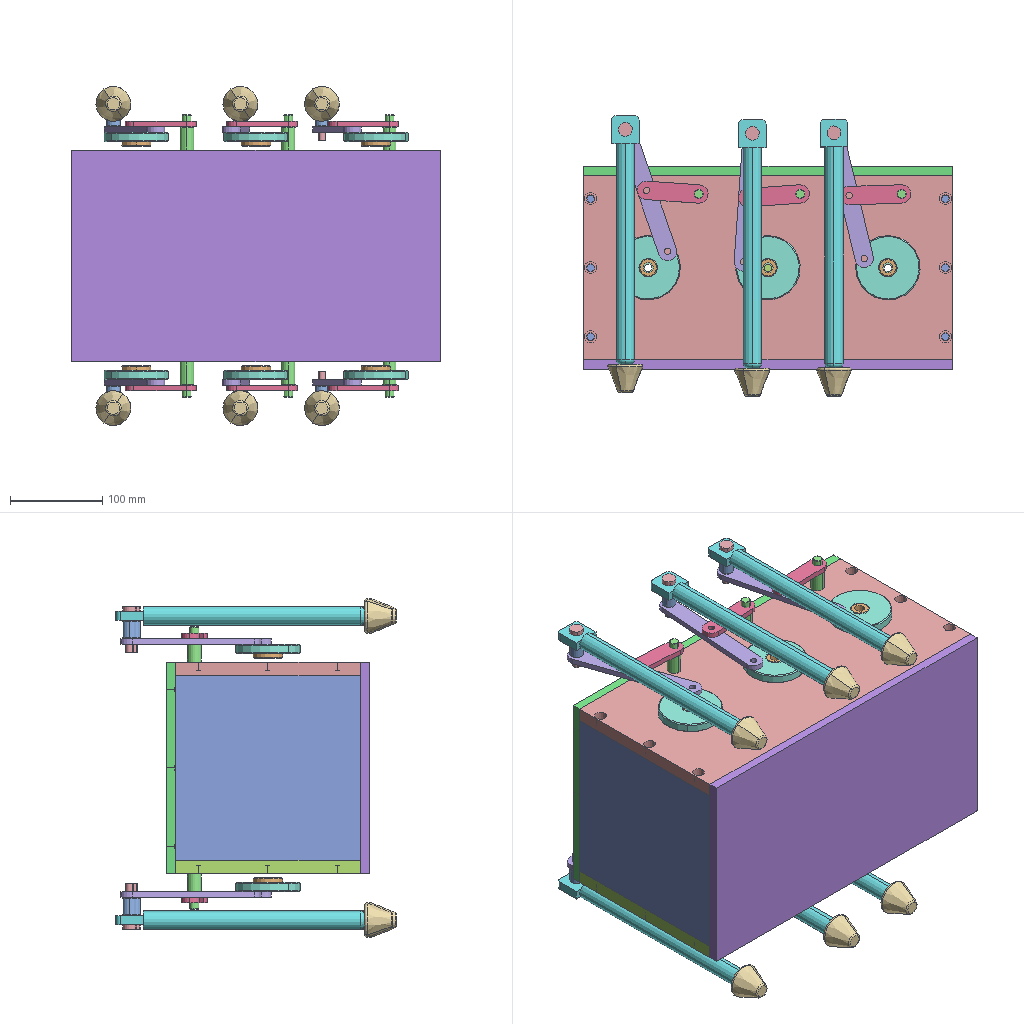Assembly | SolidWorks | 25 different items | 82 placed | box 400 x 304 x 368 mm
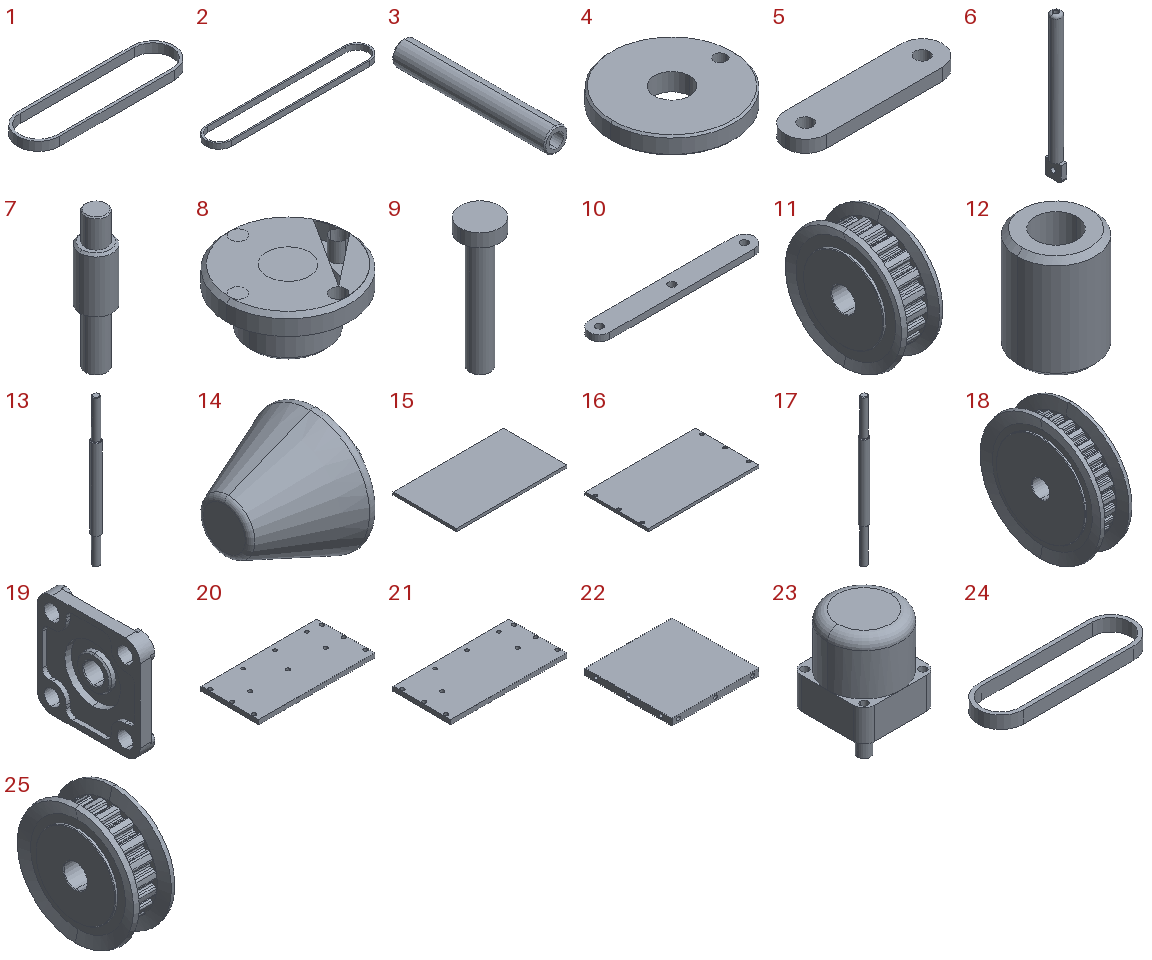Parts list (item | quantity | size | volume | features):
1 | x1 | 178 x 48 x 10 mm | 12041 mm3 | features Extrusion 1, Shell 1
2 | x1 | 308 x 48 x 10 mm | 19841 mm3 | features Extrusion 1, Shell 1
3 | x4 | 10 x 65 x 10 mm | 4498 mm3 | features Chamfer 1, Extrusion 1, HoleWzd 1, MirrorPattern 1
4 | x6 | 70 x 70 x 10 mm | 34740 mm3 | features ICE 2, Chamfer 1, Extrusion 1
5 | x6 | 77.02 x 20 x 6 mm | 8266 mm3 | features Extrusion 1, ICE 1
6 | x6 | 20 x 30 x 270 mm | 82350 mm3 | features ICE 3, Fillet 2, Extrusion 1
7 | x6 | 15 x 15 x 63 mm | 7376 mm3 | features ICE 3, Chamfer 2, Extrusion 1
8 | x6 | 32 x 32 x 15 mm | 5406 mm3 | features ICE 3, Chamfer 1, CirPattern 1, Extrusion 1
9 | x6 | 15 x 15 x 50 mm | 3143 mm3 | features Chamfer 1, Extrusion 1, ICE 1
10 | x6 | 160 x 20 x 6 mm | 17992 mm3 | features ICE 2, Extrusion 1
11 | x1 | 14 x 40 x 40 mm | 11703 mm3 | features BaseBody 1
12 | x6 | 15 x 15 x 20 mm | 2484 mm3 | features Chamfer 1, Extrusion 1, ICE 1
13 | x1 | 15 x 15 x 249 mm | 34858 mm3 | features ICE 3, Chamfer 2, Extrusion 1
14 | x6 | 40 x 38.092 x 38.092 mm | 19850 mm3 | features Fillet 2, ICE 1, Revolution 1
15 | x1 | 400 x 230 x 10 mm | 920000 mm3 | features Extrusion 1
16 | x1 | 400 x 230 x 10 mm | 912451 mm3 | features Cut 2, Extrusion 1, MirrorPattern 1
17 | x1 | 15 x 15 x 268 mm | 36663 mm3 | features ICE 3, Chamfer 2, Extrusion 1
18 | x4 | 14 x 55 x 55 mm | 22610 mm3 | features BaseBody 1
19 | x6 | 30.9 x 76 x 76 mm | 51262 mm3 | features BaseBody 1
20 | x1 | 400 x 200 x 15 mm | 1180293 mm3 | features LPattern 4, Cut 2, ICE 2, MirrorPattern 2, Extrusion 1
21 | x1 | 400 x 200 x 15 mm | 1182284 mm3 | features LPattern 4, Cut 2, ICE 2, MirrorPattern 2, Extrusion 1
22 | x2 | 200 x 200 x 15 mm | 585603 mm3 | features MirrorPattern 4, LPattern 2, Cut 1, Extrusion 1, ICE 1
23 | x1 | 70 x 70 x 121 mm | 341225 mm3 | features ICE 4, Chamfer 2, Fillet 2, CirPattern 1, Extrusion 1
24 | x1 | 124 x 36 x 10 mm | 8390 mm3 | features Extrusion 1, Shell 1
25 | x1 | 14 x 40 x 40 mm | 10988 mm3 | features BaseBody 1
Mates (type | each side: item.copy, entity, surface, feature):
Coincident | 20.1 face plane Boss-Extrude1 | 22.1 face plane Boss-Extrude1 | 3 times
Coincident | 22.2 face plane Boss-Extrude1 | 21.1 face plane Boss-Extrude1
Concentric | 22.2 face cylinder Mirror2 | 21.1 face cylinder LPattern1
Parallel | 22.2 face plane Boss-Extrude1 | 21.1 face plane Boss-Extrude1
Concentric | 21.1 face cylinder Cut-Extrude3 | 19.1 face cylinder Input1
Coincident | 21.1 face plane Boss-Extrude1 | 19.1 face plane Input1
Parallel | 22.2 face plane Boss-Extrude1 | 19.1 face plane Input1
Concentric | 13.1 face | 19.1 face cylinder Input1
Coincident | 13.1 face | 19.1 face plane Input1
Parallel | 22.2 plane | 13.1 plane
Concentric | 19.2 face cylinder Input1 | 17.1 face
Coincident | 19.2 face plane Input1 | 17.1 face
Concentric | 17.1 face | 4.1 face cylinder Boss-Extrude1
Coincident | 17.1 face | 4.1 face plane Boss-Extrude1
Concentric | 4.1 face cylinder Cut-Extrude1 | 8.1 face cylinder Boss-Extrude2
Coincident | 4.1 face plane Boss-Extrude1 | 8.1 face plane Boss-Extrude2
Parallel | 20.1 face plane Boss-Extrude1 | 8.1 plane
Concentric | 4.1 face cylinder Cut-Extrude2 | 10.1 face cylinder Cut-Extrude1
Coincident | 4.1 face plane Boss-Extrude1 | 10.1 face plane Boss-Extrude1
Concentric | 20.1 face cylinder Cut-Extrude4 | 7.1 face cylinder Boss-Extrude1
Coincident | 20.1 face plane Boss-Extrude1 | 7.1 face plane Boss-Extrude2
Parallel | 22.1 face plane Boss-Extrude1 | 7.1 plane
Concentric | 7.1 face cylinder Boss-Extrude3 | 5.1 face cylinder Cut-Extrude1
Coincident | 10.1 face plane Boss-Extrude1 | 5.1 face plane Boss-Extrude1
Concentric | 10.1 face cylinder Cut-Extrude2 | 5.1 face cylinder Cut-Extrude1
Coincident | 4.1 face plane Boss-Extrude1 | 4.2 face plane Boss-Extrude1
Concentric | 7.2 face cylinder Boss-Extrude3 | 5.2 face cylinder Cut-Extrude1
Coincident | 7.2 face plane Boss-Extrude4 | 5.2 face plane Boss-Extrude1
Concentric | 4.2 face cylinder Cut-Extrude2 | 10.2 face cylinder Cut-Extrude1
Coincident | 4.2 face plane Boss-Extrude1 | 10.2 face plane Boss-Extrude1
Concentric | 5.2 face cylinder Cut-Extrude1 | 10.2 face cylinder Cut-Extrude2
Concentric | 4.2 face cylinder Cut-Extrude1 | 8.2 face cylinder Cut-Extrude2
Coincident | 4.2 face plane Boss-Extrude1 | 8.2 face plane Boss-Extrude2
Concentric | 13.1 face | 4.3 face cylinder Cut-Extrude1
Coincident | 4.2 face plane Boss-Extrude1 | 4.3 face plane Boss-Extrude1
Concentric | 4.3 face cylinder Cut-Extrude1 | 8.3 face cylinder Boss-Extrude1
Coincident | 4.3 face plane Boss-Extrude1 | 8.3 face plane Boss-Extrude2
Parallel | 20.1 face plane Boss-Extrude1 | 13.1 plane
Concentric | 7.3 face cylinder Boss-Extrude3 | 5.3 face cylinder Cut-Extrude1
Coincident | 7.3 face plane Boss-Extrude4 | 5.3 face plane Boss-Extrude1
Concentric | 4.3 face cylinder Cut-Extrude2 | 10.3 face cylinder Cut-Extrude1
Coincident | 4.3 face plane Boss-Extrude1 | 10.3 face plane Boss-Extrude1
Concentric | 5.3 face cylinder Cut-Extrude1 | 10.3 face cylinder Cut-Extrude2
DistanceDim | 21.1 face plane Boss-Extrude1 | 23.1 face plane Boss-Extrude1 | 2 times
DistanceDim | 21.1 plane | 23.1 plane
Concentric | 23.1 face cylinder Boss-Extrude4 | 25.1 face cylinder Input1
DistanceDim | 23.1 face plane Boss-Extrude4 | 25.1 face plane Input1
Concentric | 20.1 face cylinder LPattern3 | 19.3 face cylinder Input1
Coincident | 20.1 face plane Boss-Extrude1 | 19.3 face plane Input1
Parallel | 20.1 face plane Boss-Extrude1 | 19.3 face plane Input1
Concentric | 19.3 face cylinder Input1 | 19.4 face cylinder Input1
Coincident | 21.1 face plane Boss-Extrude1 | 19.4 face plane Input1
Parallel | 21.1 face plane Boss-Extrude1 | 19.4 face plane Input1
Concentric | 8.2 face cylinder Cut-Extrude2 | 17.2 face
Coincident | 19.3 face plane Input1 | 17.2 face
Concentric | 17.2 face | 11.1 face cylinder Input1
Coincident | 25.1 face plane Input1 | 11.1 face plane Input1
Concentric | 17.2 face | 18.1 face cylinder Input1
DistanceDim | 18.1 face plane Input1 | 11.1 face plane Input1
Concentric | 13.1 face | 18.2 face cylinder Input1
Coincident | 18.1 face plane Input1 | 18.2 face plane Input1
Concentric | 13.1 face | 18.3 face cylinder Input1
DistanceDim | 19.5 face plane Input1 | 18.3 face plane Input1
Concentric | 17.1 face | 18.4 face cylinder Input1
Coincident | 18.3 face plane Input1 | 18.4 face plane Input1
Concentric | 17.2 face | 24.1 face cylinder Shell1
Coincident | 11.1 face plane Input1 | 24.1 face plane Boss-Extrude1
PlanarAngleDim | 24.1 face plane Boss-Extrude1 | 23.1 face plane Boss-Extrude1
Concentric | 18.1 face cylinder Input1 | 1.1 face cylinder Shell1
Coincident | 18.1 face plane Input1 | 1.1 face plane Boss-Extrude1
PlanarAngleDim | 1.1 face plane Boss-Extrude1 | 21.1 face plane Boss-Extrude1
Concentric | 18.4 face cylinder Input1 | 2.1 face cylinder Shell1
Coincident | 18.4 face plane Input1 | 2.1 edge
Parallel | 22.1 face plane Boss-Extrude1 | 2.1 face plane Boss-Extrude1
Concentric | 23.1 face cylinder CirPattern1 | 3.1 face cylinder Boss-Extrude1
Coincident | 21.1 face plane Boss-Extrude1 | 3.1 face plane Boss-Extrude1
Concentric | 10.1 face cylinder Cut-Extrude1 | 6.1 face cylinder Cut-Extrude1
DistanceDim | 10.1 face plane Boss-Extrude1 | 6.1 face plane Boss-Extrude2
Parallel | 22.1 face plane Boss-Extrude1 | 6.1 face plane Boss-Extrude2
Concentric | 6.1 face cylinder Boss-Extrude1 | 14.1 face cylinder Boss-Extrude1
Coincident | 6.1 face plane Boss-Extrude1 | 14.1 face plane Revolve1
Concentric | 10.2 face cylinder Cut-Extrude1 | 6.2 face cylinder Cut-Extrude1
Coincident | 6.1 face plane Boss-Extrude2 | 6.2 face plane Boss-Extrude2
Parallel | 22.1 face plane Boss-Extrude1 | 6.2 face plane Boss-Extrude2
Concentric | 10.3 face cylinder Cut-Extrude1 | 6.3 face cylinder Cut-Extrude1
Coincident | 6.1 face plane Boss-Extrude2 | 6.3 face plane Boss-Extrude2
Parallel | 22.2 face plane Boss-Extrude1 | 6.3 face plane Boss-Extrude2
Concentric | 6.2 face cylinder Boss-Extrude1 | 14.2 face cylinder Boss-Extrude1
Coincident | 6.2 face plane Boss-Extrude1 | 14.2 face plane Revolve1
Concentric | 6.3 face cylinder Boss-Extrude1 | 14.3 face cylinder Boss-Extrude1
Coincident | 6.3 face plane Boss-Extrude1 | 14.3 face plane Revolve1
Coincident | 22.1 face plane Boss-Extrude1 | 15.1 face plane Boss-Extrude1 | 2 times
Coincident | 20.1 face plane Boss-Extrude1 | 15.1 face plane Boss-Extrude1
Coincident | 20.1 face plane Boss-Extrude1 | 16.1 face plane Boss-Extrude1 | 2 times
Coincident | 22.2 face plane Boss-Extrude1 | 16.1 face plane Boss-Extrude1
Concentric | 6.4 face cylinder Cut-Extrude1 | 9.1 face cylinder Boss-Extrude1
Coincident | 6.4 face plane Boss-Extrude2 | 9.1 face plane Boss-Extrude2
Concentric | 6.5 face cylinder Cut-Extrude1 | 9.2 face cylinder Boss-Extrude1
Coincident | 9.1 face plane Boss-Extrude2 | 9.2 face plane Boss-Extrude2
Concentric | 6.6 face cylinder Cut-Extrude1 | 9.3 face cylinder Boss-Extrude1
Coincident | 6.6 face plane Boss-Extrude2 | 9.3 face plane Boss-Extrude2
Concentric | 9.4 face cylinder Boss-Extrude1 | 12.1 face cylinder Boss-Extrude1
Coincident | 10.1 face plane Boss-Extrude1 | 12.1 face plane Boss-Extrude1
Concentric | 9.5 face cylinder Boss-Extrude1 | 12.2 face cylinder Boss-Extrude1
Coincident | 6.2 face plane Boss-Extrude2 | 12.2 face plane Boss-Extrude1
Concentric | 9.6 face cylinder Boss-Extrude1 | 12.3 face cylinder Boss-Extrude1
Coincident | 10.3 face plane Boss-Extrude1 | 12.3 face plane Boss-Extrude1